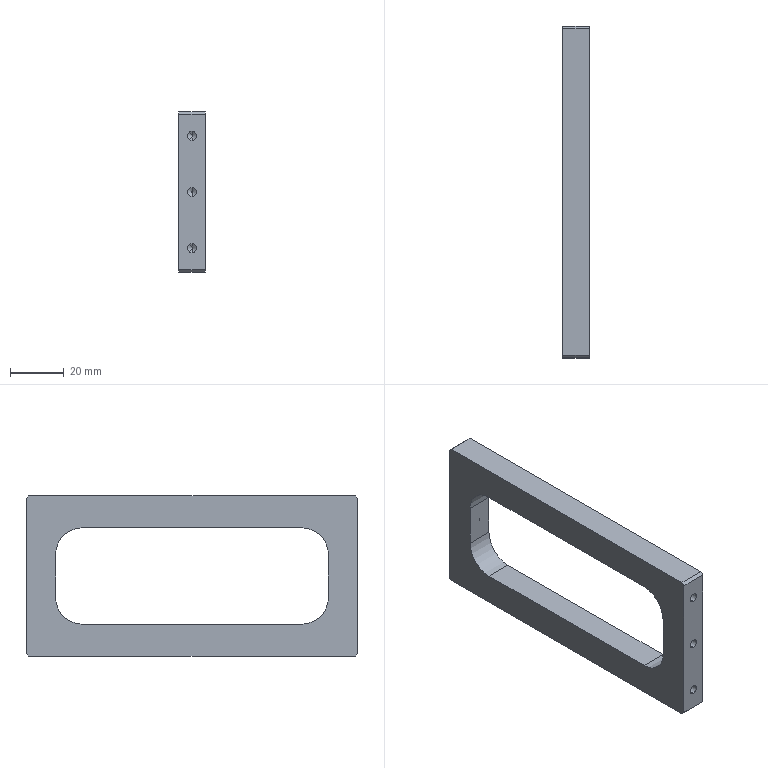Part | SolidWorks | features HoleWzd 2, Chamfer 1, Extrusion 1, Fillet 1, ICE 1 | 1 solid | 42 faces | box 10 x 124 x 60 mm | volume 37983 mm3 | cylinder 16 | plane 14 | cone 12 | commonest cylinder face diameters 3.3 x12 20 x4
STEP:
#1=CARTESIAN_POINT('',(0.,-51.9,1.65));
#2=VERTEX_POINT('',#1);
#3=CARTESIAN_POINT('',(0.,-51.9,-1.65));
#4=VERTEX_POINT('',#3);
#5=CARTESIAN_POINT('',(0.,-51.9,0.));
#6=DIRECTION('',(0.,-1.,0.));
#7=DIRECTION('',(0.,0.,-1.));
#8=AXIS2_PLACEMENT_3D('',#5,#6,#7);
#9=CIRCLE('',#8,1.65);
#10=EDGE_CURVE('',#2,#4,#9,.T.);
#11=ORIENTED_EDGE('',*,*,#10,.F.);
#12=CARTESIAN_POINT('',(0.,-62.,1.65));
#13=VERTEX_POINT('',#12);
#14=CARTESIAN_POINT('',(0.,-62.,1.65));
#15=DIRECTION('',(0.,-1.,0.));
#16=VECTOR('',#15,1000.);
#17=LINE('',#14,#16);
#18=EDGE_CURVE('',#2,#13,#17,.T.);
#19=ORIENTED_EDGE('',*,*,#18,.T.);
#20=CARTESIAN_POINT('',(0.,-62.,-1.65));
#21=VERTEX_POINT('',#20);
#22=CARTESIAN_POINT('',(0.,-62.,0.));
#23=DIRECTION('',(0.,-1.,0.));
#24=DIRECTION('',(0.,0.,-1.));
#25=AXIS2_PLACEMENT_3D('',#22,#23,#24);
#26=CIRCLE('',#25,1.65);
#27=EDGE_CURVE('',#13,#21,#26,.T.);
#28=ORIENTED_EDGE('',*,*,#27,.T.);
#29=CARTESIAN_POINT('',(0.,-62.,-1.65));
#30=DIRECTION('',(0.,-1.,0.));
#31=VECTOR('',#30,1000.);
#32=LINE('',#29,#31);
#33=EDGE_CURVE('',#4,#21,#32,.T.);
#34=ORIENTED_EDGE('',*,*,#33,.F.);
#35=EDGE_LOOP('',(#11,#19,#28,#34));
#36=FACE_OUTER_BOUND('',#35,.T.);
#37=CARTESIAN_POINT('',(0.,-62.,0.));
#38=DIRECTION('',(0.,-1.,0.));
#39=DIRECTION('',(0.,0.,-1.));
#40=AXIS2_PLACEMENT_3D('',#37,#38,#39);
#41=CYLINDRICAL_SURFACE('',#40,1.65);
#42=ADVANCED_FACE('',(#36),#41,.F.);
#43=CARTESIAN_POINT('',(0.,-51.,0.1521));
#44=VERTEX_POINT('',#43);
#45=CARTESIAN_POINT('',(0.,-51.,-0.1521));
#46=VERTEX_POINT('',#45);
#47=CARTESIAN_POINT('',(0.,-51.,0.));
#48=DIRECTION('',(0.,-1.,0.));
#49=DIRECTION('',(0.,0.,-1.));
#50=AXIS2_PLACEMENT_3D('',#47,#48,#49);
#51=CIRCLE('',#50,0.1521);
#52=EDGE_CURVE('',#44,#46,#51,.T.);
#53=ORIENTED_EDGE('',*,*,#52,.F.);
#54=CARTESIAN_POINT('',(0.,-51.9,1.65));
#55=DIRECTION('',(0.,-0.515,0.8572));
#56=VECTOR('',#55,1000.);
#57=LINE('',#54,#56);
#58=EDGE_CURVE('',#44,#2,#57,.T.);
#59=ORIENTED_EDGE('',*,*,#58,.T.);
#60=ORIENTED_EDGE('',*,*,#10,.T.);
#61=CARTESIAN_POINT('',(0.,-51.9,-1.65));
#62=DIRECTION('',(0.,-0.515,-0.8572));
#63=VECTOR('',#62,1000.);
#64=LINE('',#61,#63);
#65=EDGE_CURVE('',#46,#4,#64,.T.);
#66=ORIENTED_EDGE('',*,*,#65,.F.);
#67=EDGE_LOOP('',(#53,#59,#60,#66));
#68=FACE_OUTER_BOUND('',#67,.T.);
#69=CARTESIAN_POINT('',(0.,-51.9,0.));
#70=DIRECTION('',(0.,-1.,0.));
#71=DIRECTION('',(0.,0.,-1.));
#72=AXIS2_PLACEMENT_3D('',#69,#70,#71);
#73=CONICAL_SURFACE('',#72,1.65,1.03);
#74=ADVANCED_FACE('',(#68),#73,.F.);
#75=CARTESIAN_POINT('',(0.,-51.9,-19.35));
#76=VERTEX_POINT('',#75);
#77=CARTESIAN_POINT('',(0.,-51.9,-22.65));
#78=VERTEX_POINT('',#77);
#79=CARTESIAN_POINT('',(0.,-51.9,-21.));
#80=DIRECTION('',(0.,-1.,0.));
#81=DIRECTION('',(0.,0.,-1.));
#82=AXIS2_PLACEMENT_3D('',#79,#80,#81);
#83=CIRCLE('',#82,1.65);
#84=EDGE_CURVE('',#76,#78,#83,.T.);
#85=ORIENTED_EDGE('',*,*,#84,.F.);
#86=CARTESIAN_POINT('',(0.,-62.,-19.35));
#87=VERTEX_POINT('',#86);
#88=CARTESIAN_POINT('',(0.,-62.,-19.35));
#89=DIRECTION('',(0.,-1.,0.));
#90=VECTOR('',#89,1000.);
#91=LINE('',#88,#90);
#92=EDGE_CURVE('',#76,#87,#91,.T.);
#93=ORIENTED_EDGE('',*,*,#92,.T.);
#94=CARTESIAN_POINT('',(0.,-62.,-22.65));
#95=VERTEX_POINT('',#94);
#96=CARTESIAN_POINT('',(0.,-62.,-21.));
#97=DIRECTION('',(0.,-1.,0.));
#98=DIRECTION('',(0.,0.,-1.));
#99=AXIS2_PLACEMENT_3D('',#96,#97,#98);
#100=CIRCLE('',#99,1.65);
#101=EDGE_CURVE('',#87,#95,#100,.T.);
#102=ORIENTED_EDGE('',*,*,#101,.T.);
#103=CARTESIAN_POINT('',(0.,-62.,-22.65));
#104=DIRECTION('',(0.,-1.,0.));
#105=VECTOR('',#104,1000.);
#106=LINE('',#103,#105);
#107=EDGE_CURVE('',#78,#95,#106,.T.);
#108=ORIENTED_EDGE('',*,*,#107,.F.);
#109=EDGE_LOOP('',(#85,#93,#102,#108));
#110=FACE_OUTER_BOUND('',#109,.T.);
#111=CARTESIAN_POINT('',(0.,-62.,-21.));
#112=DIRECTION('',(0.,-1.,0.));
#113=DIRECTION('',(0.,0.,-1.));
#114=AXIS2_PLACEMENT_3D('',#111,#112,#113);
#115=CYLINDRICAL_SURFACE('',#114,1.65);
#116=ADVANCED_FACE('',(#110),#115,.F.);
#117=CARTESIAN_POINT('',(0.,-50.909,-21.));
#118=VERTEX_POINT('',#117);
#119=CARTESIAN_POINT('',(0.,-51.9,-22.65));
#120=DIRECTION('',(0.,-0.515,-0.8572));
#121=VECTOR('',#120,1000.);
#122=LINE('',#119,#121);
#123=EDGE_CURVE('',#118,#78,#122,.T.);
#124=ORIENTED_EDGE('',*,*,#123,.F.);
#125=CARTESIAN_POINT('',(0.,-51.9,-19.35));
#126=DIRECTION('',(0.,-0.515,0.8572));
#127=VECTOR('',#126,1000.);
#128=LINE('',#125,#127);
#129=EDGE_CURVE('',#118,#76,#128,.T.);
#130=ORIENTED_EDGE('',*,*,#129,.T.);
#131=ORIENTED_EDGE('',*,*,#84,.T.);
#132=EDGE_LOOP('',(#124,#130,#131));
#133=FACE_OUTER_BOUND('',#132,.T.);
#134=CARTESIAN_POINT('',(0.,-51.9,-21.));
#135=DIRECTION('',(0.,-1.,0.));
#136=DIRECTION('',(0.,0.,-1.));
#137=AXIS2_PLACEMENT_3D('',#134,#135,#136);
#138=CONICAL_SURFACE('',#137,1.65,1.03);
#139=ADVANCED_FACE('',(#133),#138,.F.);
#140=CARTESIAN_POINT('',(0.,-51.9,22.65));
#141=VERTEX_POINT('',#140);
#142=CARTESIAN_POINT('',(0.,-51.9,19.35));
#143=VERTEX_POINT('',#142);
#144=CARTESIAN_POINT('',(0.,-51.9,21.));
#145=DIRECTION('',(0.,-1.,0.));
#146=DIRECTION('',(0.,0.,-1.));
#147=AXIS2_PLACEMENT_3D('',#144,#145,#146);
#148=CIRCLE('',#147,1.65);
#149=EDGE_CURVE('',#141,#143,#148,.T.);
#150=ORIENTED_EDGE('',*,*,#149,.F.);
#151=CARTESIAN_POINT('',(0.,-62.,22.65));
#152=VERTEX_POINT('',#151);
#153=CARTESIAN_POINT('',(0.,-62.,22.65));
#154=DIRECTION('',(0.,-1.,0.));
#155=VECTOR('',#154,1000.);
#156=LINE('',#153,#155);
#157=EDGE_CURVE('',#141,#152,#156,.T.);
#158=ORIENTED_EDGE('',*,*,#157,.T.);
#159=CARTESIAN_POINT('',(0.,-62.,19.35));
#160=VERTEX_POINT('',#159);
#161=CARTESIAN_POINT('',(0.,-62.,21.));
#162=DIRECTION('',(0.,-1.,0.));
#163=DIRECTION('',(0.,0.,-1.));
#164=AXIS2_PLACEMENT_3D('',#161,#162,#163);
#165=CIRCLE('',#164,1.65);
#166=EDGE_CURVE('',#152,#160,#165,.T.);
#167=ORIENTED_EDGE('',*,*,#166,.T.);
#168=CARTESIAN_POINT('',(0.,-62.,19.35));
#169=DIRECTION('',(0.,-1.,0.));
#170=VECTOR('',#169,1000.);
#171=LINE('',#168,#170);
#172=EDGE_CURVE('',#143,#160,#171,.T.);
#173=ORIENTED_EDGE('',*,*,#172,.F.);
#174=EDGE_LOOP('',(#150,#158,#167,#173));
#175=FACE_OUTER_BOUND('',#174,.T.);
#176=CARTESIAN_POINT('',(0.,-62.,21.));
#177=DIRECTION('',(0.,-1.,0.));
#178=DIRECTION('',(0.,0.,-1.));
#179=AXIS2_PLACEMENT_3D('',#176,#177,#178);
#180=CYLINDRICAL_SURFACE('',#179,1.65);
#181=ADVANCED_FACE('',(#175),#180,.F.);
#182=CARTESIAN_POINT('',(0.,-50.909,21.));
#183=VERTEX_POINT('',#182);
#184=CARTESIAN_POINT('',(0.,-51.9,19.35));
#185=DIRECTION('',(0.,-0.515,-0.8572));
#186=VECTOR('',#185,1000.);
#187=LINE('',#184,#186);
#188=EDGE_CURVE('',#183,#143,#187,.T.);
#189=ORIENTED_EDGE('',*,*,#188,.F.);
#190=CARTESIAN_POINT('',(0.,-51.9,22.65));
#191=DIRECTION('',(0.,-0.515,0.8572));
#192=VECTOR('',#191,1000.);
#193=LINE('',#190,#192);
#194=EDGE_CURVE('',#183,#141,#193,.T.);
#195=ORIENTED_EDGE('',*,*,#194,.T.);
#196=ORIENTED_EDGE('',*,*,#149,.T.);
#197=EDGE_LOOP('',(#189,#195,#196));
#198=FACE_OUTER_BOUND('',#197,.T.);
#199=CARTESIAN_POINT('',(0.,-51.9,21.));
#200=DIRECTION('',(0.,-1.,0.));
#201=DIRECTION('',(0.,0.,-1.));
#202=AXIS2_PLACEMENT_3D('',#199,#200,#201);
#203=CONICAL_SURFACE('',#202,1.65,1.03);
#204=ADVANCED_FACE('',(#198),#203,.F.);
#205=CARTESIAN_POINT('',(0.,51.9,-1.65));
#206=VERTEX_POINT('',#205);
#207=CARTESIAN_POINT('',(0.,51.9,1.65));
#208=VERTEX_POINT('',#207);
#209=CARTESIAN_POINT('',(0.,51.9,0.));
#210=DIRECTION('',(0.,1.,0.));
#211=DIRECTION('',(0.,0.,1.));
#212=AXIS2_PLACEMENT_3D('',#209,#210,#211);
#213=CIRCLE('',#212,1.65);
#214=EDGE_CURVE('',#206,#208,#213,.T.);
#215=ORIENTED_EDGE('',*,*,#214,.F.);
#216=CARTESIAN_POINT('',(0.,62.,-1.65));
#217=VERTEX_POINT('',#216);
#218=CARTESIAN_POINT('',(0.,62.,-1.65));
#219=DIRECTION('',(0.,1.,0.));
#220=VECTOR('',#219,1000.);
#221=LINE('',#218,#220);
#222=EDGE_CURVE('',#206,#217,#221,.T.);
#223=ORIENTED_EDGE('',*,*,#222,.T.);
#224=CARTESIAN_POINT('',(0.,62.,1.65));
#225=VERTEX_POINT('',#224);
#226=CARTESIAN_POINT('',(0.,62.,0.));
#227=DIRECTION('',(0.,1.,0.));
#228=DIRECTION('',(0.,0.,1.));
#229=AXIS2_PLACEMENT_3D('',#226,#227,#228);
#230=CIRCLE('',#229,1.65);
#231=EDGE_CURVE('',#217,#225,#230,.T.);
#232=ORIENTED_EDGE('',*,*,#231,.T.);
#233=CARTESIAN_POINT('',(0.,62.,1.65));
#234=DIRECTION('',(0.,1.,0.));
#235=VECTOR('',#234,1000.);
#236=LINE('',#233,#235);
#237=EDGE_CURVE('',#208,#225,#236,.T.);
#238=ORIENTED_EDGE('',*,*,#237,.F.);
#239=EDGE_LOOP('',(#215,#223,#232,#238));
#240=FACE_OUTER_BOUND('',#239,.T.);
#241=CARTESIAN_POINT('',(0.,62.,0.));
#242=DIRECTION('',(0.,1.,0.));
#243=DIRECTION('',(0.,0.,1.));
#244=AXIS2_PLACEMENT_3D('',#241,#242,#243);
#245=CYLINDRICAL_SURFACE('',#244,1.65);
#246=ADVANCED_FACE('',(#240),#245,.F.);
#247=CARTESIAN_POINT('',(0.,51.,-0.1521));
#248=VERTEX_POINT('',#247);
#249=CARTESIAN_POINT('',(0.,51.,0.1521));
#250=VERTEX_POINT('',#249);
#251=CARTESIAN_POINT('',(0.,51.,0.));
#252=DIRECTION('',(0.,1.,0.));
#253=DIRECTION('',(0.,0.,1.));
#254=AXIS2_PLACEMENT_3D('',#251,#252,#253);
#255=CIRCLE('',#254,0.1521);
#256=EDGE_CURVE('',#248,#250,#255,.T.);
#257=ORIENTED_EDGE('',*,*,#256,.F.);
#258=CARTESIAN_POINT('',(0.,51.9,-1.65));
#259=DIRECTION('',(0.,0.515,-0.8572));
#260=VECTOR('',#259,1000.);
#261=LINE('',#258,#260);
#262=EDGE_CURVE('',#248,#206,#261,.T.);
#263=ORIENTED_EDGE('',*,*,#262,.T.);
#264=ORIENTED_EDGE('',*,*,#214,.T.);
#265=CARTESIAN_POINT('',(0.,51.9,1.65));
#266=DIRECTION('',(0.,0.515,0.8572));
#267=VECTOR('',#266,1000.);
#268=LINE('',#265,#267);
#269=EDGE_CURVE('',#250,#208,#268,.T.);
#270=ORIENTED_EDGE('',*,*,#269,.F.);
#271=EDGE_LOOP('',(#257,#263,#264,#270));
#272=FACE_OUTER_BOUND('',#271,.T.);
#273=CARTESIAN_POINT('',(0.,51.9,0.));
#274=DIRECTION('',(0.,1.,0.));
#275=DIRECTION('',(0.,0.,1.));
#276=AXIS2_PLACEMENT_3D('',#273,#274,#275);
#277=CONICAL_SURFACE('',#276,1.65,1.03);
#278=ADVANCED_FACE('',(#272),#277,.F.);
#279=CARTESIAN_POINT('',(0.,51.9,-22.65));
#280=VERTEX_POINT('',#279);
#281=CARTESIAN_POINT('',(0.,51.9,-19.35));
#282=VERTEX_POINT('',#281);
#283=CARTESIAN_POINT('',(0.,51.9,-21.));
#284=DIRECTION('',(0.,1.,0.));
#285=DIRECTION('',(0.,0.,1.));
#286=AXIS2_PLACEMENT_3D('',#283,#284,#285);
#287=CIRCLE('',#286,1.65);
#288=EDGE_CURVE('',#280,#282,#287,.T.);
#289=ORIENTED_EDGE('',*,*,#288,.F.);
#290=CARTESIAN_POINT('',(0.,62.,-22.65));
#291=VERTEX_POINT('',#290);
#292=CARTESIAN_POINT('',(0.,62.,-22.65));
#293=DIRECTION('',(0.,1.,0.));
#294=VECTOR('',#293,1000.);
#295=LINE('',#292,#294);
#296=EDGE_CURVE('',#280,#291,#295,.T.);
#297=ORIENTED_EDGE('',*,*,#296,.T.);
#298=CARTESIAN_POINT('',(0.,62.,-19.35));
#299=VERTEX_POINT('',#298);
#300=CARTESIAN_POINT('',(0.,62.,-21.));
#301=DIRECTION('',(0.,1.,0.));
#302=DIRECTION('',(0.,0.,1.));
#303=AXIS2_PLACEMENT_3D('',#300,#301,#302);
#304=CIRCLE('',#303,1.65);
#305=EDGE_CURVE('',#291,#299,#304,.T.);
#306=ORIENTED_EDGE('',*,*,#305,.T.);
#307=CARTESIAN_POINT('',(0.,62.,-19.35));
#308=DIRECTION('',(0.,1.,0.));
#309=VECTOR('',#308,1000.);
#310=LINE('',#307,#309);
#311=EDGE_CURVE('',#282,#299,#310,.T.);
#312=ORIENTED_EDGE('',*,*,#311,.F.);
#313=EDGE_LOOP('',(#289,#297,#306,#312));
#314=FACE_OUTER_BOUND('',#313,.T.);
#315=CARTESIAN_POINT('',(0.,62.,-21.));
#316=DIRECTION('',(0.,1.,0.));
#317=DIRECTION('',(0.,0.,1.));
#318=AXIS2_PLACEMENT_3D('',#315,#316,#317);
#319=CYLINDRICAL_SURFACE('',#318,1.65);
#320=ADVANCED_FACE('',(#314),#319,.F.);
#321=CARTESIAN_POINT('',(0.,50.909,-21.));
#322=VERTEX_POINT('',#321);
#323=CARTESIAN_POINT('',(0.,51.9,-19.35));
#324=DIRECTION('',(0.,0.515,0.8572));
#325=VECTOR('',#324,1000.);
#326=LINE('',#323,#325);
#327=EDGE_CURVE('',#322,#282,#326,.T.);
#328=ORIENTED_EDGE('',*,*,#327,.F.);
#329=CARTESIAN_POINT('',(0.,51.9,-22.65));
#330=DIRECTION('',(0.,0.515,-0.8572));
#331=VECTOR('',#330,1000.);
#332=LINE('',#329,#331);
#333=EDGE_CURVE('',#322,#280,#332,.T.);
#334=ORIENTED_EDGE('',*,*,#333,.T.);
#335=ORIENTED_EDGE('',*,*,#288,.T.);
#336=EDGE_LOOP('',(#328,#334,#335));
#337=FACE_OUTER_BOUND('',#336,.T.);
#338=CARTESIAN_POINT('',(0.,51.9,-21.));
#339=DIRECTION('',(0.,1.,0.));
#340=DIRECTION('',(0.,0.,1.));
#341=AXIS2_PLACEMENT_3D('',#338,#339,#340);
#342=CONICAL_SURFACE('',#341,1.65,1.03);
#343=ADVANCED_FACE('',(#337),#342,.F.);
#344=CARTESIAN_POINT('',(0.,51.9,19.35));
#345=VERTEX_POINT('',#344);
#346=CARTESIAN_POINT('',(0.,51.9,22.65));
#347=VERTEX_POINT('',#346);
#348=CARTESIAN_POINT('',(0.,51.9,21.));
#349=DIRECTION('',(0.,1.,0.));
#350=DIRECTION('',(0.,0.,1.));
#351=AXIS2_PLACEMENT_3D('',#348,#349,#350);
#352=CIRCLE('',#351,1.65);
#353=EDGE_CURVE('',#345,#347,#352,.T.);
#354=ORIENTED_EDGE('',*,*,#353,.F.);
#355=CARTESIAN_POINT('',(0.,62.,19.35));
#356=VERTEX_POINT('',#355);
#357=CARTESIAN_POINT('',(0.,62.,19.35));
#358=DIRECTION('',(0.,1.,0.));
#359=VECTOR('',#358,1000.);
#360=LINE('',#357,#359);
#361=EDGE_CURVE('',#345,#356,#360,.T.);
#362=ORIENTED_EDGE('',*,*,#361,.T.);
#363=CARTESIAN_POINT('',(0.,62.,22.65));
#364=VERTEX_POINT('',#363);
#365=CARTESIAN_POINT('',(0.,62.,21.));
#366=DIRECTION('',(0.,1.,0.));
#367=DIRECTION('',(0.,0.,1.));
#368=AXIS2_PLACEMENT_3D('',#365,#366,#367);
#369=CIRCLE('',#368,1.65);
#370=EDGE_CURVE('',#356,#364,#369,.T.);
#371=ORIENTED_EDGE('',*,*,#370,.T.);
#372=CARTESIAN_POINT('',(0.,62.,22.65));
#373=DIRECTION('',(0.,1.,0.));
#374=VECTOR('',#373,1000.);
#375=LINE('',#372,#374);
#376=EDGE_CURVE('',#347,#364,#375,.T.);
#377=ORIENTED_EDGE('',*,*,#376,.F.);
#378=EDGE_LOOP('',(#354,#362,#371,#377));
#379=FACE_OUTER_BOUND('',#378,.T.);
#380=CARTESIAN_POINT('',(0.,62.,21.));
#381=DIRECTION('',(0.,1.,0.));
#382=DIRECTION('',(0.,0.,1.));
#383=AXIS2_PLACEMENT_3D('',#380,#381,#382);
#384=CYLINDRICAL_SURFACE('',#383,1.65);
#385=ADVANCED_FACE('',(#379),#384,.F.);
#386=CARTESIAN_POINT('',(0.,50.909,21.));
#387=VERTEX_POINT('',#386);
#388=CARTESIAN_POINT('',(0.,51.9,22.65));
#389=DIRECTION('',(0.,0.515,0.8572));
#390=VECTOR('',#389,1000.);
#391=LINE('',#388,#390);
#392=EDGE_CURVE('',#387,#347,#391,.T.);
#393=ORIENTED_EDGE('',*,*,#392,.F.);
#394=CARTESIAN_POINT('',(0.,51.9,19.35));
#395=DIRECTION('',(0.,0.515,-0.8572));
#396=VECTOR('',#395,1000.);
#397=LINE('',#394,#396);
#398=EDGE_CURVE('',#387,#345,#397,.T.);
#399=ORIENTED_EDGE('',*,*,#398,.T.);
#400=ORIENTED_EDGE('',*,*,#353,.T.);
#401=EDGE_LOOP('',(#393,#399,#400));
#402=FACE_OUTER_BOUND('',#401,.T.);
#403=CARTESIAN_POINT('',(0.,51.9,21.));
#404=DIRECTION('',(0.,1.,0.));
#405=DIRECTION('',(0.,0.,1.));
#406=AXIS2_PLACEMENT_3D('',#403,#404,#405);
#407=CONICAL_SURFACE('',#406,1.65,1.03);
#408=ADVANCED_FACE('',(#402),#407,.F.);
#409=CARTESIAN_POINT('',(0.,-62.,-21.));
#410=DIRECTION('',(0.,-1.,0.));
#411=DIRECTION('',(0.,0.,-1.));
#412=AXIS2_PLACEMENT_3D('',#409,#410,#411);
#413=CIRCLE('',#412,1.65);
#414=EDGE_CURVE('',#95,#87,#413,.T.);
#415=ORIENTED_EDGE('',*,*,#414,.F.);
#416=ORIENTED_EDGE('',*,*,#101,.F.);
#417=EDGE_LOOP('',(#415,#416));
#418=FACE_BOUND('',#417,.T.);
#419=CARTESIAN_POINT('',(0.,-62.,21.));
#420=DIRECTION('',(0.,-1.,0.));
#421=DIRECTION('',(0.,0.,-1.));
#422=AXIS2_PLACEMENT_3D('',#419,#420,#421);
#423=CIRCLE('',#422,1.65);
#424=EDGE_CURVE('',#160,#152,#423,.T.);
#425=ORIENTED_EDGE('',*,*,#424,.F.);
#426=ORIENTED_EDGE('',*,*,#166,.F.);
#427=EDGE_LOOP('',(#425,#426));
#428=FACE_BOUND('',#427,.T.);
#429=CARTESIAN_POINT('',(-5.,-62.,29.));
#430=VERTEX_POINT('',#429);
#431=CARTESIAN_POINT('',(-5.,-62.,-29.));
#432=VERTEX_POINT('',#431);
#433=CARTESIAN_POINT('',(-5.,-62.,30.));
#434=DIRECTION('',(0.,0.,-1.));
#435=VECTOR('',#434,1000.);
#436=LINE('',#433,#435);
#437=EDGE_CURVE('',#430,#432,#436,.T.);
#438=ORIENTED_EDGE('',*,*,#437,.T.);
#439=CARTESIAN_POINT('',(5.,-62.,-29.));
#440=VERTEX_POINT('',#439);
#441=CARTESIAN_POINT('',(5.,-62.,-29.));
#442=DIRECTION('',(1.,0.,0.));
#443=VECTOR('',#442,1000.);
#444=LINE('',#441,#443);
#445=EDGE_CURVE('',#432,#440,#444,.T.);
#446=ORIENTED_EDGE('',*,*,#445,.T.);
#447=CARTESIAN_POINT('',(5.,-62.,29.));
#448=VERTEX_POINT('',#447);
#449=CARTESIAN_POINT('',(5.,-62.,30.));
#450=DIRECTION('',(0.,0.,-1.));
#451=VECTOR('',#450,1000.);
#452=LINE('',#449,#451);
#453=EDGE_CURVE('',#448,#440,#452,.T.);
#454=ORIENTED_EDGE('',*,*,#453,.F.);
#455=CARTESIAN_POINT('',(5.,-62.,29.));
#456=DIRECTION('',(-1.,0.,0.));
#457=VECTOR('',#456,1000.);
#458=LINE('',#455,#457);
#459=EDGE_CURVE('',#448,#430,#458,.T.);
#460=ORIENTED_EDGE('',*,*,#459,.T.);
#461=EDGE_LOOP('',(#438,#446,#454,#460));
#462=FACE_OUTER_BOUND('',#461,.T.);
#463=CARTESIAN_POINT('',(0.,-62.,0.));
#464=DIRECTION('',(0.,-1.,0.));
#465=DIRECTION('',(0.,0.,-1.));
#466=AXIS2_PLACEMENT_3D('',#463,#464,#465);
#467=CIRCLE('',#466,1.65);
#468=EDGE_CURVE('',#21,#13,#467,.T.);
#469=ORIENTED_EDGE('',*,*,#468,.F.);
#470=ORIENTED_EDGE('',*,*,#27,.F.);
#471=EDGE_LOOP('',(#469,#470));
#472=FACE_BOUND('',#471,.T.);
#473=CARTESIAN_POINT('',(5.,-62.,30.));
#474=DIRECTION('',(0.,1.,0.));
#475=DIRECTION('',(0.,0.,1.));
#476=AXIS2_PLACEMENT_3D('',#473,#474,#475);
#477=PLANE('',#476);
#478=ADVANCED_FACE('',(#418,#428,#462,#472),#477,.F.);
#479=CARTESIAN_POINT('',(5.,-61.,-30.));
#480=VERTEX_POINT('',#479);
#481=CARTESIAN_POINT('',(5.,61.,-30.));
#482=VERTEX_POINT('',#481);
#483=CARTESIAN_POINT('',(5.,62.,-30.));
#484=DIRECTION('',(0.,1.,0.));
#485=VECTOR('',#484,1000.);
#486=LINE('',#483,#485);
#487=EDGE_CURVE('',#480,#482,#486,.T.);
#488=ORIENTED_EDGE('',*,*,#487,.F.);
#489=CARTESIAN_POINT('',(-5.,-61.,-30.));
#490=VERTEX_POINT('',#489);
#491=CARTESIAN_POINT('',(5.,-61.,-30.));
#492=DIRECTION('',(-1.,0.,0.));
#493=VECTOR('',#492,1000.);
#494=LINE('',#491,#493);
#495=EDGE_CURVE('',#480,#490,#494,.T.);
#496=ORIENTED_EDGE('',*,*,#495,.T.);
#497=CARTESIAN_POINT('',(-5.,61.,-30.));
#498=VERTEX_POINT('',#497);
#499=CARTESIAN_POINT('',(-5.,62.,-30.));
#500=DIRECTION('',(0.,1.,0.));
#501=VECTOR('',#500,1000.);
#502=LINE('',#499,#501);
#503=EDGE_CURVE('',#490,#498,#502,.T.);
#504=ORIENTED_EDGE('',*,*,#503,.T.);
#505=CARTESIAN_POINT('',(5.,61.,-30.));
#506=DIRECTION('',(1.,0.,0.));
#507=VECTOR('',#506,1000.);
#508=LINE('',#505,#507);
#509=EDGE_CURVE('',#498,#482,#508,.T.);
#510=ORIENTED_EDGE('',*,*,#509,.T.);
#511=EDGE_LOOP('',(#488,#496,#504,#510));
#512=FACE_OUTER_BOUND('',#511,.T.);
#513=CARTESIAN_POINT('',(5.,62.,-30.));
#514=DIRECTION('',(0.,0.,1.));
#515=DIRECTION('',(0.,-1.,0.));
#516=AXIS2_PLACEMENT_3D('',#513,#514,#515);
#517=PLANE('',#516);
#518=ADVANCED_FACE('',(#512),#517,.F.);
#519=CARTESIAN_POINT('',(0.,62.,0.));
#520=DIRECTION('',(0.,1.,0.));
#521=DIRECTION('',(0.,0.,1.));
#522=AXIS2_PLACEMENT_3D('',#519,#520,#521);
#523=CIRCLE('',#522,1.65);
#524=EDGE_CURVE('',#225,#217,#523,.T.);
#525=ORIENTED_EDGE('',*,*,#524,.F.);
#526=ORIENTED_EDGE('',*,*,#231,.F.);
#527=EDGE_LOOP('',(#525,#526));
#528=FACE_BOUND('',#527,.T.);
#529=CARTESIAN_POINT('',(0.,62.,-21.));
#530=DIRECTION('',(0.,1.,0.));
#531=DIRECTION('',(0.,0.,1.));
#532=AXIS2_PLACEMENT_3D('',#529,#530,#531);
#533=CIRCLE('',#532,1.65);
#534=EDGE_CURVE('',#299,#291,#533,.T.);
#535=ORIENTED_EDGE('',*,*,#534,.F.);
#536=ORIENTED_EDGE('',*,*,#305,.F.);
#537=EDGE_LOOP('',(#535,#536));
#538=FACE_BOUND('',#537,.T.);
#539=CARTESIAN_POINT('',(0.,62.,21.));
#540=DIRECTION('',(0.,1.,0.));
#541=DIRECTION('',(0.,0.,1.));
#542=AXIS2_PLACEMENT_3D('',#539,#540,#541);
#543=CIRCLE('',#542,1.65);
#544=EDGE_CURVE('',#364,#356,#543,.T.);
#545=ORIENTED_EDGE('',*,*,#544,.F.);
#546=ORIENTED_EDGE('',*,*,#370,.F.);
#547=EDGE_LOOP('',(#545,#546));
#548=FACE_BOUND('',#547,.T.);
#549=CARTESIAN_POINT('',(5.,62.,-29.));
#550=VERTEX_POINT('',#549);
#551=CARTESIAN_POINT('',(5.,62.,29.));
#552=VERTEX_POINT('',#551);
#553=CARTESIAN_POINT('',(5.,62.,30.));
#554=DIRECTION('',(0.,0.,1.));
#555=VECTOR('',#554,1000.);
#556=LINE('',#553,#555);
#557=EDGE_CURVE('',#550,#552,#556,.T.);
#558=ORIENTED_EDGE('',*,*,#557,.F.);
#559=CARTESIAN_POINT('',(-5.,62.,-29.));
#560=VERTEX_POINT('',#559);
#561=CARTESIAN_POINT('',(5.,62.,-29.));
#562=DIRECTION('',(-1.,0.,0.));
#563=VECTOR('',#562,1000.);
#564=LINE('',#561,#563);
#565=EDGE_CURVE('',#550,#560,#564,.T.);
#566=ORIENTED_EDGE('',*,*,#565,.T.);
#567=CARTESIAN_POINT('',(-5.,62.,29.));
#568=VERTEX_POINT('',#567);
#569=CARTESIAN_POINT('',(-5.,62.,30.));
#570=DIRECTION('',(0.,0.,1.));
#571=VECTOR('',#570,1000.);
#572=LINE('',#569,#571);
#573=EDGE_CURVE('',#560,#568,#572,.T.);
#574=ORIENTED_EDGE('',*,*,#573,.T.);
#575=CARTESIAN_POINT('',(5.,62.,29.));
#576=DIRECTION('',(1.,0.,0.));
#577=VECTOR('',#576,1000.);
#578=LINE('',#575,#577);
#579=EDGE_CURVE('',#568,#552,#578,.T.);
#580=ORIENTED_EDGE('',*,*,#579,.T.);
#581=EDGE_LOOP('',(#558,#566,#574,#580));
#582=FACE_OUTER_BOUND('',#581,.T.);
#583=CARTESIAN_POINT('',(5.,62.,30.));
#584=DIRECTION('',(0.,-1.,0.));
#585=DIRECTION('',(0.,0.,-1.));
#586=AXIS2_PLACEMENT_3D('',#583,#584,#585);
#587=PLANE('',#586);
#588=ADVANCED_FACE('',(#528,#538,#548,#582),#587,.F.);
#589=CARTESIAN_POINT('',(-5.,61.,30.));
#590=VERTEX_POINT('',#589);
#591=CARTESIAN_POINT('',(-5.,-61.,30.));
#592=VERTEX_POINT('',#591);
#593=CARTESIAN_POINT('',(-5.,62.,30.));
#594=DIRECTION('',(0.,-1.,0.));
#595=VECTOR('',#594,1000.);
#596=LINE('',#593,#595);
#597=EDGE_CURVE('',#590,#592,#596,.T.);
#598=ORIENTED_EDGE('',*,*,#597,.T.);
#599=CARTESIAN_POINT('',(5.,-61.,30.));
#600=VERTEX_POINT('',#599);
#601=CARTESIAN_POINT('',(5.,-61.,30.));
#602=DIRECTION('',(1.,0.,0.));
#603=VECTOR('',#602,1000.);
#604=LINE('',#601,#603);
#605=EDGE_CURVE('',#592,#600,#604,.T.);
#606=ORIENTED_EDGE('',*,*,#605,.T.);
#607=CARTESIAN_POINT('',(5.,61.,30.));
#608=VERTEX_POINT('',#607);
#609=CARTESIAN_POINT('',(5.,62.,30.));
#610=DIRECTION('',(0.,-1.,0.));
#611=VECTOR('',#610,1000.);
#612=LINE('',#609,#611);
#613=EDGE_CURVE('',#608,#600,#612,.T.);
#614=ORIENTED_EDGE('',*,*,#613,.F.);
#615=CARTESIAN_POINT('',(5.,61.,30.));
#616=DIRECTION('',(-1.,0.,0.));
#617=VECTOR('',#616,1000.);
#618=LINE('',#615,#617);
#619=EDGE_CURVE('',#608,#590,#618,.T.);
#620=ORIENTED_EDGE('',*,*,#619,.T.);
#621=EDGE_LOOP('',(#598,#606,#614,#620));
#622=FACE_OUTER_BOUND('',#621,.T.);
#623=CARTESIAN_POINT('',(5.,62.,30.));
#624=DIRECTION('',(0.,0.,-1.));
#625=DIRECTION('',(0.,1.,0.));
#626=AXIS2_PLACEMENT_3D('',#623,#624,#625);
#627=PLANE('',#626);
#628=ADVANCED_FACE('',(#622),#627,.F.);
#629=CARTESIAN_POINT('',(5.,-41.,-18.));
#630=VERTEX_POINT('',#629);
#631=CARTESIAN_POINT('',(5.,41.,-18.));
#632=VERTEX_POINT('',#631);
#633=CARTESIAN_POINT('',(5.,51.,-18.));
#634=DIRECTION('',(0.,1.,0.));
#635=VECTOR('',#634,1000.);
#636=LINE('',#633,#635);
#637=EDGE_CURVE('',#630,#632,#636,.T.);
#638=ORIENTED_EDGE('',*,*,#637,.F.);
#639=CARTESIAN_POINT('',(5.,-51.,-8.));
#640=VERTEX_POINT('',#639);
#641=CARTESIAN_POINT('',(5.,-41.,-8.));
#642=DIRECTION('',(-1.,0.,0.));
#643=DIRECTION('',(0.,0.,-1.));
#644=AXIS2_PLACEMENT_3D('',#641,#642,#643);
#645=CIRCLE('',#644,10.);
#646=EDGE_CURVE('',#630,#640,#645,.T.);
#647=ORIENTED_EDGE('',*,*,#646,.T.);
#648=CARTESIAN_POINT('',(5.,-51.,8.));
#649=VERTEX_POINT('',#648);
#650=CARTESIAN_POINT('',(5.,-51.,18.));
#651=DIRECTION('',(0.,0.,-1.));
#652=VECTOR('',#651,1000.);
#653=LINE('',#650,#652);
#654=EDGE_CURVE('',#649,#640,#653,.T.);
#655=ORIENTED_EDGE('',*,*,#654,.F.);
#656=CARTESIAN_POINT('',(5.,-41.,18.));
#657=VERTEX_POINT('',#656);
#658=CARTESIAN_POINT('',(5.,-41.,8.));
#659=DIRECTION('',(-1.,0.,0.));
#660=DIRECTION('',(0.,0.,-1.));
#661=AXIS2_PLACEMENT_3D('',#658,#659,#660);
#662=CIRCLE('',#661,10.);
#663=EDGE_CURVE('',#649,#657,#662,.T.);
#664=ORIENTED_EDGE('',*,*,#663,.T.);
#665=CARTESIAN_POINT('',(5.,41.,18.));
#666=VERTEX_POINT('',#665);
#667=CARTESIAN_POINT('',(5.,51.,18.));
#668=DIRECTION('',(0.,-1.,0.));
#669=VECTOR('',#668,1000.);
#670=LINE('',#667,#669);
#671=EDGE_CURVE('',#666,#657,#670,.T.);
#672=ORIENTED_EDGE('',*,*,#671,.F.);
#673=CARTESIAN_POINT('',(5.,51.,8.));
#674=VERTEX_POINT('',#673);
#675=CARTESIAN_POINT('',(5.,41.,8.));
#676=DIRECTION('',(-1.,0.,0.));
#677=DIRECTION('',(0.,0.,-1.));
#678=AXIS2_PLACEMENT_3D('',#675,#676,#677);
#679=CIRCLE('',#678,10.);
#680=EDGE_CURVE('',#666,#674,#679,.T.);
#681=ORIENTED_EDGE('',*,*,#680,.T.);
#682=CARTESIAN_POINT('',(5.,51.,-8.));
#683=VERTEX_POINT('',#682);
#684=CARTESIAN_POINT('',(5.,51.,18.));
#685=DIRECTION('',(0.,0.,1.));
#686=VECTOR('',#685,1000.);
#687=LINE('',#684,#686);
#688=EDGE_CURVE('',#683,#674,#687,.T.);
#689=ORIENTED_EDGE('',*,*,#688,.F.);
#690=CARTESIAN_POINT('',(5.,41.,-8.));
#691=DIRECTION('',(-1.,0.,0.));
#692=DIRECTION('',(0.,0.,-1.));
#693=AXIS2_PLACEMENT_3D('',#690,#691,#692);
#694=CIRCLE('',#693,10.);
#695=EDGE_CURVE('',#683,#632,#694,.T.);
#696=ORIENTED_EDGE('',*,*,#695,.T.);
#697=EDGE_LOOP('',(#638,#647,#655,#664,#672,#681,#689,#696));
#698=FACE_BOUND('',#697,.T.);
#699=ORIENTED_EDGE('',*,*,#453,.T.);
#700=CARTESIAN_POINT('',(5.,-45.5,-45.5));
#701=DIRECTION('',(0.,0.7071,-0.7071));
#702=VECTOR('',#701,1000.);
#703=LINE('',#700,#702);
#704=EDGE_CURVE('',#440,#480,#703,.T.);
#705=ORIENTED_EDGE('',*,*,#704,.T.);
#706=ORIENTED_EDGE('',*,*,#487,.T.);
#707=CARTESIAN_POINT('',(5.,45.5,-45.5));
#708=DIRECTION('',(0.,0.7071,0.7071));
#709=VECTOR('',#708,1000.);
#710=LINE('',#707,#709);
#711=EDGE_CURVE('',#482,#550,#710,.T.);
#712=ORIENTED_EDGE('',*,*,#711,.T.);
#713=ORIENTED_EDGE('',*,*,#557,.T.);
#714=CARTESIAN_POINT('',(5.,45.5,45.5));
#715=DIRECTION('',(0.,-0.7071,0.7071));
#716=VECTOR('',#715,1000.);
#717=LINE('',#714,#716);
#718=EDGE_CURVE('',#552,#608,#717,.T.);
#719=ORIENTED_EDGE('',*,*,#718,.T.);
#720=ORIENTED_EDGE('',*,*,#613,.T.);
#721=CARTESIAN_POINT('',(5.,-45.5,45.5));
#722=DIRECTION('',(0.,-0.7071,-0.7071));
#723=VECTOR('',#722,1000.);
#724=LINE('',#721,#723);
#725=EDGE_CURVE('',#600,#448,#724,.T.);
#726=ORIENTED_EDGE('',*,*,#725,.T.);
#727=EDGE_LOOP('',(#699,#705,#706,#712,#713,#719,#720,#726));
#728=FACE_OUTER_BOUND('',#727,.T.);
#729=CARTESIAN_POINT('',(5.,0.,0.));
#730=DIRECTION('',(1.,0.,0.));
#731=DIRECTION('',(0.,0.,-1.));
#732=AXIS2_PLACEMENT_3D('',#729,#730,#731);
#733=PLANE('',#732);
#734=ADVANCED_FACE('',(#698,#728),#733,.T.);
#735=CARTESIAN_POINT('',(-5.,41.,18.));
#736=VERTEX_POINT('',#735);
#737=CARTESIAN_POINT('',(-5.,-41.,18.));
#738=VERTEX_POINT('',#737);
#739=CARTESIAN_POINT('',(-5.,51.,18.));
#740=DIRECTION('',(0.,-1.,0.));
#741=VECTOR('',#740,1000.);
#742=LINE('',#739,#741);
#743=EDGE_CURVE('',#736,#738,#742,.T.);
#744=ORIENTED_EDGE('',*,*,#743,.T.);
#745=CARTESIAN_POINT('',(-5.,-51.,8.));
#746=VERTEX_POINT('',#745);
#747=CARTESIAN_POINT('',(-5.,-41.,8.));
#748=DIRECTION('',(1.,0.,0.));
#749=DIRECTION('',(0.,0.,-1.));
#750=AXIS2_PLACEMENT_3D('',#747,#748,#749);
#751=CIRCLE('',#750,10.);
#752=EDGE_CURVE('',#738,#746,#751,.T.);
#753=ORIENTED_EDGE('',*,*,#752,.T.);
#754=CARTESIAN_POINT('',(-5.,-51.,-8.));
#755=VERTEX_POINT('',#754);
#756=CARTESIAN_POINT('',(-5.,-51.,18.));
#757=DIRECTION('',(0.,0.,-1.));
#758=VECTOR('',#757,1000.);
#759=LINE('',#756,#758);
#760=EDGE_CURVE('',#746,#755,#759,.T.);
#761=ORIENTED_EDGE('',*,*,#760,.T.);
#762=CARTESIAN_POINT('',(-5.,-41.,-18.));
#763=VERTEX_POINT('',#762);
#764=CARTESIAN_POINT('',(-5.,-41.,-8.));
#765=DIRECTION('',(1.,0.,0.));
#766=DIRECTION('',(0.,0.,-1.));
#767=AXIS2_PLACEMENT_3D('',#764,#765,#766);
#768=CIRCLE('',#767,10.);
#769=EDGE_CURVE('',#755,#763,#768,.T.);
#770=ORIENTED_EDGE('',*,*,#769,.T.);
#771=CARTESIAN_POINT('',(-5.,41.,-18.));
#772=VERTEX_POINT('',#771);
#773=CARTESIAN_POINT('',(-5.,51.,-18.));
#774=DIRECTION('',(0.,1.,0.));
#775=VECTOR('',#774,1000.);
#776=LINE('',#773,#775);
#777=EDGE_CURVE('',#763,#772,#776,.T.);
#778=ORIENTED_EDGE('',*,*,#777,.T.);
#779=CARTESIAN_POINT('',(-5.,51.,-8.));
#780=VERTEX_POINT('',#779);
#781=CARTESIAN_POINT('',(-5.,41.,-8.));
#782=DIRECTION('',(1.,0.,0.));
#783=DIRECTION('',(0.,0.,-1.));
#784=AXIS2_PLACEMENT_3D('',#781,#782,#783);
#785=CIRCLE('',#784,10.);
#786=EDGE_CURVE('',#772,#780,#785,.T.);
#787=ORIENTED_EDGE('',*,*,#786,.T.);
#788=CARTESIAN_POINT('',(-5.,51.,8.));
#789=VERTEX_POINT('',#788);
#790=CARTESIAN_POINT('',(-5.,51.,18.));
#791=DIRECTION('',(0.,0.,1.));
#792=VECTOR('',#791,1000.);
#793=LINE('',#790,#792);
#794=EDGE_CURVE('',#780,#789,#793,.T.);
#795=ORIENTED_EDGE('',*,*,#794,.T.);
#796=CARTESIAN_POINT('',(-5.,41.,8.));
#797=DIRECTION('',(1.,0.,0.));
#798=DIRECTION('',(0.,0.,-1.));
#799=AXIS2_PLACEMENT_3D('',#796,#797,#798);
#800=CIRCLE('',#799,10.);
#801=EDGE_CURVE('',#789,#736,#800,.T.);
#802=ORIENTED_EDGE('',*,*,#801,.T.);
#803=EDGE_LOOP('',(#744,#753,#761,#770,#778,#787,#795,#802));
#804=FACE_BOUND('',#803,.T.);
#805=ORIENTED_EDGE('',*,*,#503,.F.);
#806=CARTESIAN_POINT('',(-5.,-61.,-30.));
#807=DIRECTION('',(0.,-0.7071,0.7071));
#808=VECTOR('',#807,1000.);
#809=LINE('',#806,#808);
#810=EDGE_CURVE('',#490,#432,#809,.T.);
#811=ORIENTED_EDGE('',*,*,#810,.T.);
#812=ORIENTED_EDGE('',*,*,#437,.F.);
#813=CARTESIAN_POINT('',(-5.,-62.,29.));
#814=DIRECTION('',(0.,0.7071,0.7071));
#815=VECTOR('',#814,1000.);
#816=LINE('',#813,#815);
#817=EDGE_CURVE('',#430,#592,#816,.T.);
#818=ORIENTED_EDGE('',*,*,#817,.T.);
#819=ORIENTED_EDGE('',*,*,#597,.F.);
#820=CARTESIAN_POINT('',(-5.,61.,30.));
#821=DIRECTION('',(0.,0.7071,-0.7071));
#822=VECTOR('',#821,1000.);
#823=LINE('',#820,#822);
#824=EDGE_CURVE('',#590,#568,#823,.T.);
#825=ORIENTED_EDGE('',*,*,#824,.T.);
#826=ORIENTED_EDGE('',*,*,#573,.F.);
#827=CARTESIAN_POINT('',(-5.,62.,-29.));
#828=DIRECTION('',(0.,-0.7071,-0.7071));
#829=VECTOR('',#828,1000.);
#830=LINE('',#827,#829);
#831=EDGE_CURVE('',#560,#498,#830,.T.);
#832=ORIENTED_EDGE('',*,*,#831,.T.);
#833=EDGE_LOOP('',(#805,#811,#812,#818,#819,#825,#826,#832));
#834=FACE_OUTER_BOUND('',#833,.T.);
#835=CARTESIAN_POINT('',(-5.,0.,0.));
#836=DIRECTION('',(1.,0.,0.));
#837=DIRECTION('',(0.,0.,-1.));
#838=AXIS2_PLACEMENT_3D('',#835,#836,#837);
#839=PLANE('',#838);
#840=ADVANCED_FACE('',(#804,#834),#839,.F.);
#841=ORIENTED_EDGE('',*,*,#777,.F.);
#842=CARTESIAN_POINT('',(5.,-41.,-18.));
#843=DIRECTION('',(1.,0.,0.));
#844=VECTOR('',#843,1000.);
#845=LINE('',#842,#844);
#846=EDGE_CURVE('',#763,#630,#845,.T.);
#847=ORIENTED_EDGE('',*,*,#846,.T.);
#848=ORIENTED_EDGE('',*,*,#637,.T.);
#849=CARTESIAN_POINT('',(-5.,41.,-18.));
#850=DIRECTION('',(-1.,0.,0.));
#851=VECTOR('',#850,1000.);
#852=LINE('',#849,#851);
#853=EDGE_CURVE('',#632,#772,#852,.T.);
#854=ORIENTED_EDGE('',*,*,#853,.T.);
#855=EDGE_LOOP('',(#841,#847,#848,#854));
#856=FACE_OUTER_BOUND('',#855,.T.);
#857=CARTESIAN_POINT('',(-5.,51.,-18.));
#858=DIRECTION('',(0.,0.,-1.));
#859=DIRECTION('',(0.,1.,0.));
#860=AXIS2_PLACEMENT_3D('',#857,#858,#859);
#861=PLANE('',#860);
#862=ADVANCED_FACE('',(#856),#861,.F.);
#863=CARTESIAN_POINT('',(0.,-51.,0.));
#864=DIRECTION('',(0.,-1.,0.));
#865=DIRECTION('',(0.,0.,-1.));
#866=AXIS2_PLACEMENT_3D('',#863,#864,#865);
#867=CIRCLE('',#866,0.1521);
#868=EDGE_CURVE('',#46,#44,#867,.T.);
#869=ORIENTED_EDGE('',*,*,#868,.T.);
#870=ORIENTED_EDGE('',*,*,#52,.T.);
#871=EDGE_LOOP('',(#869,#870));
#872=FACE_BOUND('',#871,.T.);
#873=ORIENTED_EDGE('',*,*,#760,.F.);
#874=CARTESIAN_POINT('',(5.,-51.,8.));
#875=DIRECTION('',(1.,0.,0.));
#876=VECTOR('',#875,1000.);
#877=LINE('',#874,#876);
#878=EDGE_CURVE('',#746,#649,#877,.T.);
#879=ORIENTED_EDGE('',*,*,#878,.T.);
#880=ORIENTED_EDGE('',*,*,#654,.T.);
#881=CARTESIAN_POINT('',(-5.,-51.,-8.));
#882=DIRECTION('',(-1.,0.,0.));
#883=VECTOR('',#882,1000.);
#884=LINE('',#881,#883);
#885=EDGE_CURVE('',#640,#755,#884,.T.);
#886=ORIENTED_EDGE('',*,*,#885,.T.);
#887=EDGE_LOOP('',(#873,#879,#880,#886));
#888=FACE_OUTER_BOUND('',#887,.T.);
#889=CARTESIAN_POINT('',(-5.,-51.,18.));
#890=DIRECTION('',(0.,-1.,0.));
#891=DIRECTION('',(0.,0.,-1.));
#892=AXIS2_PLACEMENT_3D('',#889,#890,#891);
#893=PLANE('',#892);
#894=ADVANCED_FACE('',(#872,#888),#893,.F.);
#895=ORIENTED_EDGE('',*,*,#671,.T.);
#896=CARTESIAN_POINT('',(-5.,-41.,18.));
#897=DIRECTION('',(-1.,0.,0.));
#898=VECTOR('',#897,1000.);
#899=LINE('',#896,#898);
#900=EDGE_CURVE('',#657,#738,#899,.T.);
#901=ORIENTED_EDGE('',*,*,#900,.T.);
#902=ORIENTED_EDGE('',*,*,#743,.F.);
#903=CARTESIAN_POINT('',(5.,41.,18.));
#904=DIRECTION('',(1.,0.,0.));
#905=VECTOR('',#904,1000.);
#906=LINE('',#903,#905);
#907=EDGE_CURVE('',#736,#666,#906,.T.);
#908=ORIENTED_EDGE('',*,*,#907,.T.);
#909=EDGE_LOOP('',(#895,#901,#902,#908));
#910=FACE_OUTER_BOUND('',#909,.T.);
#911=CARTESIAN_POINT('',(-5.,51.,18.));
#912=DIRECTION('',(0.,0.,1.));
#913=DIRECTION('',(0.,-1.,0.));
#914=AXIS2_PLACEMENT_3D('',#911,#912,#913);
#915=PLANE('',#914);
#916=ADVANCED_FACE('',(#910),#915,.F.);
#917=CARTESIAN_POINT('',(0.,51.,0.));
#918=DIRECTION('',(0.,1.,0.));
#919=DIRECTION('',(0.,0.,1.));
#920=AXIS2_PLACEMENT_3D('',#917,#918,#919);
#921=CIRCLE('',#920,0.1521);
#922=EDGE_CURVE('',#250,#248,#921,.T.);
#923=ORIENTED_EDGE('',*,*,#922,.T.);
#924=ORIENTED_EDGE('',*,*,#256,.T.);
#925=EDGE_LOOP('',(#923,#924));
#926=FACE_BOUND('',#925,.T.);
#927=ORIENTED_EDGE('',*,*,#794,.F.);
#928=CARTESIAN_POINT('',(5.,51.,-8.));
#929=DIRECTION('',(1.,0.,0.));
#930=VECTOR('',#929,1000.);
#931=LINE('',#928,#930);
#932=EDGE_CURVE('',#780,#683,#931,.T.);
#933=ORIENTED_EDGE('',*,*,#932,.T.);
#934=ORIENTED_EDGE('',*,*,#688,.T.);
#935=CARTESIAN_POINT('',(-5.,51.,8.));
#936=DIRECTION('',(-1.,0.,0.));
#937=VECTOR('',#936,1000.);
#938=LINE('',#935,#937);
#939=EDGE_CURVE('',#674,#789,#938,.T.);
#940=ORIENTED_EDGE('',*,*,#939,.T.);
#941=EDGE_LOOP('',(#927,#933,#934,#940));
#942=FACE_OUTER_BOUND('',#941,.T.);
#943=CARTESIAN_POINT('',(-5.,51.,18.));
#944=DIRECTION('',(0.,1.,0.));
#945=DIRECTION('',(0.,0.,1.));
#946=AXIS2_PLACEMENT_3D('',#943,#944,#945);
#947=PLANE('',#946);
#948=ADVANCED_FACE('',(#926,#942),#947,.F.);
#949=ORIENTED_EDGE('',*,*,#398,.F.);
#950=ORIENTED_EDGE('',*,*,#392,.T.);
#951=CARTESIAN_POINT('',(0.,51.9,21.));
#952=DIRECTION('',(0.,1.,0.));
#953=DIRECTION('',(0.,0.,1.));
#954=AXIS2_PLACEMENT_3D('',#951,#952,#953);
#955=CIRCLE('',#954,1.65);
#956=EDGE_CURVE('',#347,#345,#955,.T.);
#957=ORIENTED_EDGE('',*,*,#956,.T.);
#958=EDGE_LOOP('',(#949,#950,#957));
#959=FACE_OUTER_BOUND('',#958,.T.);
#960=CARTESIAN_POINT('',(0.,51.9,21.));
#961=DIRECTION('',(0.,1.,0.));
#962=DIRECTION('',(0.,0.,1.));
#963=AXIS2_PLACEMENT_3D('',#960,#961,#962);
#964=CONICAL_SURFACE('',#963,1.65,1.03);
#965=ADVANCED_FACE('',(#959),#964,.F.);
#966=ORIENTED_EDGE('',*,*,#361,.F.);
#967=ORIENTED_EDGE('',*,*,#956,.F.);
#968=ORIENTED_EDGE('',*,*,#376,.T.);
#969=ORIENTED_EDGE('',*,*,#544,.T.);
#970=EDGE_LOOP('',(#966,#967,#968,#969));
#971=FACE_OUTER_BOUND('',#970,.T.);
#972=CARTESIAN_POINT('',(0.,62.,21.));
#973=DIRECTION('',(0.,1.,0.));
#974=DIRECTION('',(0.,0.,1.));
#975=AXIS2_PLACEMENT_3D('',#972,#973,#974);
#976=CYLINDRICAL_SURFACE('',#975,1.65);
#977=ADVANCED_FACE('',(#971),#976,.F.);
#978=ORIENTED_EDGE('',*,*,#333,.F.);
#979=ORIENTED_EDGE('',*,*,#327,.T.);
#980=CARTESIAN_POINT('',(0.,51.9,-21.));
#981=DIRECTION('',(0.,1.,0.));
#982=DIRECTION('',(0.,0.,1.));
#983=AXIS2_PLACEMENT_3D('',#980,#981,#982);
#984=CIRCLE('',#983,1.65);
#985=EDGE_CURVE('',#282,#280,#984,.T.);
#986=ORIENTED_EDGE('',*,*,#985,.T.);
#987=EDGE_LOOP('',(#978,#979,#986));
#988=FACE_OUTER_BOUND('',#987,.T.);
#989=CARTESIAN_POINT('',(0.,51.9,-21.));
#990=DIRECTION('',(0.,1.,0.));
#991=DIRECTION('',(0.,0.,1.));
#992=AXIS2_PLACEMENT_3D('',#989,#990,#991);
#993=CONICAL_SURFACE('',#992,1.65,1.03);
#994=ADVANCED_FACE('',(#988),#993,.F.);
#995=ORIENTED_EDGE('',*,*,#296,.F.);
#996=ORIENTED_EDGE('',*,*,#985,.F.);
#997=ORIENTED_EDGE('',*,*,#311,.T.);
#998=ORIENTED_EDGE('',*,*,#534,.T.);
#999=EDGE_LOOP('',(#995,#996,#997,#998));
#1000=FACE_OUTER_BOUND('',#999,.T.);
#1001=CARTESIAN_POINT('',(0.,62.,-21.));
#1002=DIRECTION('',(0.,1.,0.));
#1003=DIRECTION('',(0.,0.,1.));
#1004=AXIS2_PLACEMENT_3D('',#1001,#1002,#1003);
#1005=CYLINDRICAL_SURFACE('',#1004,1.65);
#1006=ADVANCED_FACE('',(#1000),#1005,.F.);
#1007=ORIENTED_EDGE('',*,*,#262,.F.);
#1008=ORIENTED_EDGE('',*,*,#922,.F.);
#1009=ORIENTED_EDGE('',*,*,#269,.T.);
#1010=CARTESIAN_POINT('',(0.,51.9,0.));
#1011=DIRECTION('',(0.,1.,0.));
#1012=DIRECTION('',(0.,0.,1.));
#1013=AXIS2_PLACEMENT_3D('',#1010,#1011,#1012);
#1014=CIRCLE('',#1013,1.65);
#1015=EDGE_CURVE('',#208,#206,#1014,.T.);
#1016=ORIENTED_EDGE('',*,*,#1015,.T.);
#1017=EDGE_LOOP('',(#1007,#1008,#1009,#1016));
#1018=FACE_OUTER_BOUND('',#1017,.T.);
#1019=CARTESIAN_POINT('',(0.,51.9,0.));
#1020=DIRECTION('',(0.,1.,0.));
#1021=DIRECTION('',(0.,0.,1.));
#1022=AXIS2_PLACEMENT_3D('',#1019,#1020,#1021);
#1023=CONICAL_SURFACE('',#1022,1.65,1.03);
#1024=ADVANCED_FACE('',(#1018),#1023,.F.);
#1025=ORIENTED_EDGE('',*,*,#222,.F.);
#1026=ORIENTED_EDGE('',*,*,#1015,.F.);
#1027=ORIENTED_EDGE('',*,*,#237,.T.);
#1028=ORIENTED_EDGE('',*,*,#524,.T.);
#1029=EDGE_LOOP('',(#1025,#1026,#1027,#1028));
#1030=FACE_OUTER_BOUND('',#1029,.T.);
#1031=CARTESIAN_POINT('',(0.,62.,0.));
#1032=DIRECTION('',(0.,1.,0.));
#1033=DIRECTION('',(0.,0.,1.));
#1034=AXIS2_PLACEMENT_3D('',#1031,#1032,#1033);
#1035=CYLINDRICAL_SURFACE('',#1034,1.65);
#1036=ADVANCED_FACE('',(#1030),#1035,.F.);
#1037=ORIENTED_EDGE('',*,*,#752,.F.);
#1038=ORIENTED_EDGE('',*,*,#900,.F.);
#1039=ORIENTED_EDGE('',*,*,#663,.F.);
#1040=ORIENTED_EDGE('',*,*,#878,.F.);
#1041=EDGE_LOOP('',(#1037,#1038,#1039,#1040));
#1042=FACE_OUTER_BOUND('',#1041,.T.);
#1043=CARTESIAN_POINT('',(-5.,-41.,8.));
#1044=DIRECTION('',(-1.,0.,0.));
#1045=DIRECTION('',(0.,0.,1.));
#1046=AXIS2_PLACEMENT_3D('',#1043,#1044,#1045);
#1047=CYLINDRICAL_SURFACE('',#1046,10.);
#1048=ADVANCED_FACE('',(#1042),#1047,.F.);
#1049=ORIENTED_EDGE('',*,*,#769,.F.);
#1050=ORIENTED_EDGE('',*,*,#885,.F.);
#1051=ORIENTED_EDGE('',*,*,#646,.F.);
#1052=ORIENTED_EDGE('',*,*,#846,.F.);
#1053=EDGE_LOOP('',(#1049,#1050,#1051,#1052));
#1054=FACE_OUTER_BOUND('',#1053,.T.);
#1055=CARTESIAN_POINT('',(-5.,-41.,-8.));
#1056=DIRECTION('',(-1.,0.,0.));
#1057=DIRECTION('',(0.,0.,1.));
#1058=AXIS2_PLACEMENT_3D('',#1055,#1056,#1057);
#1059=CYLINDRICAL_SURFACE('',#1058,10.);
#1060=ADVANCED_FACE('',(#1054),#1059,.F.);
#1061=ORIENTED_EDGE('',*,*,#786,.F.);
#1062=ORIENTED_EDGE('',*,*,#853,.F.);
#1063=ORIENTED_EDGE('',*,*,#695,.F.);
#1064=ORIENTED_EDGE('',*,*,#932,.F.);
#1065=EDGE_LOOP('',(#1061,#1062,#1063,#1064));
#1066=FACE_OUTER_BOUND('',#1065,.T.);
#1067=CARTESIAN_POINT('',(-5.,41.,-8.));
#1068=DIRECTION('',(-1.,0.,0.));
#1069=DIRECTION('',(0.,0.,1.));
#1070=AXIS2_PLACEMENT_3D('',#1067,#1068,#1069);
#1071=CYLINDRICAL_SURFACE('',#1070,10.);
#1072=ADVANCED_FACE('',(#1066),#1071,.F.);
#1073=ORIENTED_EDGE('',*,*,#801,.F.);
#1074=ORIENTED_EDGE('',*,*,#939,.F.);
#1075=ORIENTED_EDGE('',*,*,#680,.F.);
#1076=ORIENTED_EDGE('',*,*,#907,.F.);
#1077=EDGE_LOOP('',(#1073,#1074,#1075,#1076));
#1078=FACE_OUTER_BOUND('',#1077,.T.);
#1079=CARTESIAN_POINT('',(-5.,41.,8.));
#1080=DIRECTION('',(-1.,0.,0.));
#1081=DIRECTION('',(0.,0.,1.));
#1082=AXIS2_PLACEMENT_3D('',#1079,#1080,#1081);
#1083=CYLINDRICAL_SURFACE('',#1082,10.);
#1084=ADVANCED_FACE('',(#1078),#1083,.F.);
#1085=ORIENTED_EDGE('',*,*,#194,.F.);
#1086=ORIENTED_EDGE('',*,*,#188,.T.);
#1087=CARTESIAN_POINT('',(0.,-51.9,21.));
#1088=DIRECTION('',(0.,-1.,0.));
#1089=DIRECTION('',(0.,0.,-1.));
#1090=AXIS2_PLACEMENT_3D('',#1087,#1088,#1089);
#1091=CIRCLE('',#1090,1.65);
#1092=EDGE_CURVE('',#143,#141,#1091,.T.);
#1093=ORIENTED_EDGE('',*,*,#1092,.T.);
#1094=EDGE_LOOP('',(#1085,#1086,#1093));
#1095=FACE_OUTER_BOUND('',#1094,.T.);
#1096=CARTESIAN_POINT('',(0.,-51.9,21.));
#1097=DIRECTION('',(0.,-1.,0.));
#1098=DIRECTION('',(0.,0.,-1.));
#1099=AXIS2_PLACEMENT_3D('',#1096,#1097,#1098);
#1100=CONICAL_SURFACE('',#1099,1.65,1.03);
#1101=ADVANCED_FACE('',(#1095),#1100,.F.);
#1102=ORIENTED_EDGE('',*,*,#157,.F.);
#1103=ORIENTED_EDGE('',*,*,#1092,.F.);
#1104=ORIENTED_EDGE('',*,*,#172,.T.);
#1105=ORIENTED_EDGE('',*,*,#424,.T.);
#1106=EDGE_LOOP('',(#1102,#1103,#1104,#1105));
#1107=FACE_OUTER_BOUND('',#1106,.T.);
#1108=CARTESIAN_POINT('',(0.,-62.,21.));
#1109=DIRECTION('',(0.,-1.,0.));
#1110=DIRECTION('',(0.,0.,-1.));
#1111=AXIS2_PLACEMENT_3D('',#1108,#1109,#1110);
#1112=CYLINDRICAL_SURFACE('',#1111,1.65);
#1113=ADVANCED_FACE('',(#1107),#1112,.F.);
#1114=ORIENTED_EDGE('',*,*,#129,.F.);
#1115=ORIENTED_EDGE('',*,*,#123,.T.);
#1116=CARTESIAN_POINT('',(0.,-51.9,-21.));
#1117=DIRECTION('',(0.,-1.,0.));
#1118=DIRECTION('',(0.,0.,-1.));
#1119=AXIS2_PLACEMENT_3D('',#1116,#1117,#1118);
#1120=CIRCLE('',#1119,1.65);
#1121=EDGE_CURVE('',#78,#76,#1120,.T.);
#1122=ORIENTED_EDGE('',*,*,#1121,.T.);
#1123=EDGE_LOOP('',(#1114,#1115,#1122));
#1124=FACE_OUTER_BOUND('',#1123,.T.);
#1125=CARTESIAN_POINT('',(0.,-51.9,-21.));
#1126=DIRECTION('',(0.,-1.,0.));
#1127=DIRECTION('',(0.,0.,-1.));
#1128=AXIS2_PLACEMENT_3D('',#1125,#1126,#1127);
#1129=CONICAL_SURFACE('',#1128,1.65,1.03);
#1130=ADVANCED_FACE('',(#1124),#1129,.F.);
#1131=ORIENTED_EDGE('',*,*,#92,.F.);
#1132=ORIENTED_EDGE('',*,*,#1121,.F.);
#1133=ORIENTED_EDGE('',*,*,#107,.T.);
#1134=ORIENTED_EDGE('',*,*,#414,.T.);
#1135=EDGE_LOOP('',(#1131,#1132,#1133,#1134));
#1136=FACE_OUTER_BOUND('',#1135,.T.);
#1137=CARTESIAN_POINT('',(0.,-62.,-21.));
#1138=DIRECTION('',(0.,-1.,0.));
#1139=DIRECTION('',(0.,0.,-1.));
#1140=AXIS2_PLACEMENT_3D('',#1137,#1138,#1139);
#1141=CYLINDRICAL_SURFACE('',#1140,1.65);
#1142=ADVANCED_FACE('',(#1136),#1141,.F.);
#1143=ORIENTED_EDGE('',*,*,#58,.F.);
#1144=ORIENTED_EDGE('',*,*,#868,.F.);
#1145=ORIENTED_EDGE('',*,*,#65,.T.);
#1146=CARTESIAN_POINT('',(0.,-51.9,0.));
#1147=DIRECTION('',(0.,-1.,0.));
#1148=DIRECTION('',(0.,0.,-1.));
#1149=AXIS2_PLACEMENT_3D('',#1146,#1147,#1148);
#1150=CIRCLE('',#1149,1.65);
#1151=EDGE_CURVE('',#4,#2,#1150,.T.);
#1152=ORIENTED_EDGE('',*,*,#1151,.T.);
#1153=EDGE_LOOP('',(#1143,#1144,#1145,#1152));
#1154=FACE_OUTER_BOUND('',#1153,.T.);
#1155=CARTESIAN_POINT('',(0.,-51.9,0.));
#1156=DIRECTION('',(0.,-1.,0.));
#1157=DIRECTION('',(0.,0.,-1.));
#1158=AXIS2_PLACEMENT_3D('',#1155,#1156,#1157);
#1159=CONICAL_SURFACE('',#1158,1.65,1.03);
#1160=ADVANCED_FACE('',(#1154),#1159,.F.);
#1161=ORIENTED_EDGE('',*,*,#18,.F.);
#1162=ORIENTED_EDGE('',*,*,#1151,.F.);
#1163=ORIENTED_EDGE('',*,*,#33,.T.);
#1164=ORIENTED_EDGE('',*,*,#468,.T.);
#1165=EDGE_LOOP('',(#1161,#1162,#1163,#1164));
#1166=FACE_OUTER_BOUND('',#1165,.T.);
#1167=CARTESIAN_POINT('',(0.,-62.,0.));
#1168=DIRECTION('',(0.,-1.,0.));
#1169=DIRECTION('',(0.,0.,-1.));
#1170=AXIS2_PLACEMENT_3D('',#1167,#1168,#1169);
#1171=CYLINDRICAL_SURFACE('',#1170,1.65);
#1172=ADVANCED_FACE('',(#1166),#1171,.F.);
#1173=ORIENTED_EDGE('',*,*,#704,.F.);
#1174=ORIENTED_EDGE('',*,*,#445,.F.);
#1175=ORIENTED_EDGE('',*,*,#810,.F.);
#1176=ORIENTED_EDGE('',*,*,#495,.F.);
#1177=EDGE_LOOP('',(#1173,#1174,#1175,#1176));
#1178=FACE_OUTER_BOUND('',#1177,.T.);
#1179=CARTESIAN_POINT('',(5.,-61.,-30.));
#1180=DIRECTION('',(0.,0.7071,0.7071));
#1181=DIRECTION('',(-1.,0.,0.));
#1182=AXIS2_PLACEMENT_3D('',#1179,#1180,#1181);
#1183=PLANE('',#1182);
#1184=ADVANCED_FACE('',(#1178),#1183,.F.);
#1185=ORIENTED_EDGE('',*,*,#725,.F.);
#1186=ORIENTED_EDGE('',*,*,#605,.F.);
#1187=ORIENTED_EDGE('',*,*,#817,.F.);
#1188=ORIENTED_EDGE('',*,*,#459,.F.);
#1189=EDGE_LOOP('',(#1185,#1186,#1187,#1188));
#1190=FACE_OUTER_BOUND('',#1189,.T.);
#1191=CARTESIAN_POINT('',(5.,-62.,29.));
#1192=DIRECTION('',(0.,0.7071,-0.7071));
#1193=DIRECTION('',(-1.,0.,0.));
#1194=AXIS2_PLACEMENT_3D('',#1191,#1192,#1193);
#1195=PLANE('',#1194);
#1196=ADVANCED_FACE('',(#1190),#1195,.F.);
#1197=ORIENTED_EDGE('',*,*,#711,.F.);
#1198=ORIENTED_EDGE('',*,*,#509,.F.);
#1199=ORIENTED_EDGE('',*,*,#831,.F.);
#1200=ORIENTED_EDGE('',*,*,#565,.F.);
#1201=EDGE_LOOP('',(#1197,#1198,#1199,#1200));
#1202=FACE_OUTER_BOUND('',#1201,.T.);
#1203=CARTESIAN_POINT('',(5.,62.,-29.));
#1204=DIRECTION('',(0.,-0.7071,0.7071));
#1205=DIRECTION('',(-1.,0.,0.));
#1206=AXIS2_PLACEMENT_3D('',#1203,#1204,#1205);
#1207=PLANE('',#1206);
#1208=ADVANCED_FACE('',(#1202),#1207,.F.);
#1209=ORIENTED_EDGE('',*,*,#718,.F.);
#1210=ORIENTED_EDGE('',*,*,#579,.F.);
#1211=ORIENTED_EDGE('',*,*,#824,.F.);
#1212=ORIENTED_EDGE('',*,*,#619,.F.);
#1213=EDGE_LOOP('',(#1209,#1210,#1211,#1212));
#1214=FACE_OUTER_BOUND('',#1213,.T.);
#1215=CARTESIAN_POINT('',(5.,61.,30.));
#1216=DIRECTION('',(0.,-0.7071,-0.7071));
#1217=DIRECTION('',(-1.,0.,0.));
#1218=AXIS2_PLACEMENT_3D('',#1215,#1216,#1217);
#1219=PLANE('',#1218);
#1220=ADVANCED_FACE('',(#1214),#1219,.F.);
#1221=CLOSED_SHELL('',(#42,#74,#116,#139,#181,#204,#246,#278,#320,#343,#385,#408,#478,#518,#588,#628,#734,#840,#862,#894,#916,#948,#965,#977,#994,#1006,#1024,#1036,#1048,#1060,#1072,#1084,#1101,#1113,#1130,#1142,#1160,#1172,#1184,#1196,#1208,#1220));
#1222=MANIFOLD_SOLID_BREP('',#1221);
#1223=CARTESIAN_POINT('',(0.,0.,0.));
#1224=DIRECTION('',(0.,0.,1.));
#1225=DIRECTION('',(1.,0.,0.));
#1226=AXIS2_PLACEMENT_3D('',#1223,#1224,#1225);
#1227=(LENGTH_UNIT()NAMED_UNIT(*)SI_UNIT(.MILLI.,.METRE.));
#1228=UNCERTAINTY_MEASURE_WITH_UNIT(LENGTH_MEASURE(0.00001),#1227,'','');
#1229=(NAMED_UNIT(*)PLANE_ANGLE_UNIT()SI_UNIT($,.RADIAN.));
#1230=(NAMED_UNIT(*)SI_UNIT($,.STERADIAN.)SOLID_ANGLE_UNIT());
#1231=(GEOMETRIC_REPRESENTATION_CONTEXT(3)GLOBAL_UNCERTAINTY_ASSIGNED_CONTEXT((#1228))GLOBAL_UNIT_ASSIGNED_CONTEXT((#1227,#1229,#1230))REPRESENTATION_CONTEXT('',''));
#1232=ADVANCED_BREP_SHAPE_REPRESENTATION('',(#1222,#1226),#1231);